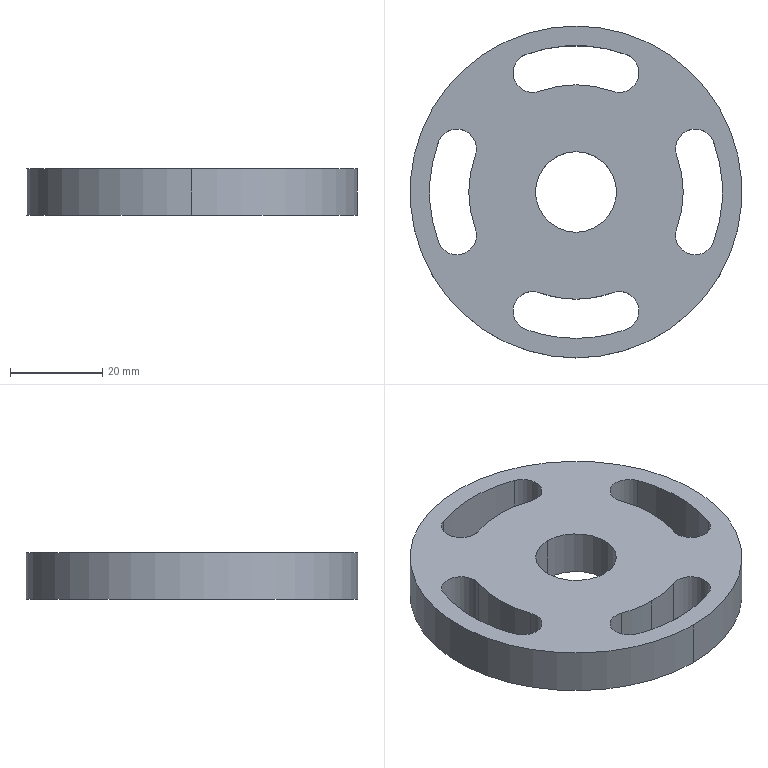NC program | NX | posted with a generic post | part box 72 x 72 x 10 mm
Lines 1 to 834 of 21342:
N10 G17 G21 G94 G90
(ZLEVEL_PROFILE , TOOL : D6C)
N12 T06 M6
N14 G54
N16 G17 G0 G90 X-6.398 Y25.475 S4000 M3
N18 G43 Z30. H6
N20 Z1.5
N22 G94 G1 X-4.667 Y25.852 Z1.407 F1800.
N24 X-2.81 Y26.119 Z1.309
N26 X-0.938 Y26.253 Z1.21
N28 X0.938 Z1.112
N30 X2.81 Y26.119 Z1.014
N32 X4.667 Y25.852 Z0.915
N34 X6.5 Y25.453 Z0.817
N36 X8.3 Y24.924 Z0.719
N38 X9.13 Y24.622 Z0.673
N40 X9.247 Y24.602 Z0.666
N42 X9.563 Y24.601 Z0.65
N44 X9.967 Y24.725 Z0.628
N46 X10.308 Y24.976 Z0.605
N48 X10.545 Y25.327 Z0.583
N50 X10.651 Y25.736 Z0.561
N52 X10.615 Y26.158 Z0.539
N54 X10.497 Y26.45 Z0.522
N56 X10.275 Y26.74 Z0.503
N58 X9.978 Y26.953 Z0.484
N60 X9.117 Y27.266 Z0.436
N62 X7.074 Y27.866 Z0.325
N64 X4.992 Y28.313 Z0.213
N66 X2.883 Y28.605 Z0.101
N68 X0.758 Y28.74 Z-0.01
N70 X0. Z-0.05
N72 G3 X-9.83 Y27.007 R28.74
N74 X-10.571 Y25.417 R1.24
N76 X-8.981 Y24.676 R1.24
N78 G2 X8.981 Y24.676 R26.26
N80 G3 X10.571 Y25.417 R1.24
N82 X9.83 Y27.007 R1.24
N84 X0. Y28.74 R28.74
N86 G1 X-0.159 Y28.736 Z-0.053
N88 X-0.318 Y28.732 Z-0.056
N90 X-0.477 Y28.728 Z-0.058
N92 X-0.636 Y28.724 Z-0.061
N94 X-0.795 Y28.72 Z-0.064
N96 X-0.954 Y28.716 Z-0.067
N98 X-1.113 Y28.712 Z-0.069
N100 X-1.273 Y28.708 Z-0.072
N102 X-1.432 Y28.704 Z-0.075
N104 X-1.59 Y28.692 Z-0.078
N106 X-1.749 Y28.681 Z-0.081
N108 X-1.908 Y28.669 Z-0.083
N110 X-2.066 Y28.657 Z-0.086
N112 X-2.225 Y28.645 Z-0.089
N114 X-2.384 Y28.633 Z-0.092
N116 X-2.542 Y28.621 Z-0.094
N118 X-2.701 Y28.609 Z-0.097
N120 X-2.86 Y28.597 Z-0.1
N122 G3 X-9.83 Y27.007 R28.74
N124 X-10.571 Y25.417 R1.24
N126 X-8.981 Y24.676 R1.24
N128 G2 X8.981 Y24.676 R26.26
N130 G3 X10.571 Y25.417 R1.24
N132 X9.83 Y27.007 R1.24
N134 X0. Y28.74 R28.74
N136 G1 X-0.159 Y28.736 Z-0.103
N138 X-0.318 Y28.732 Z-0.106
N140 X-0.477 Y28.728 Z-0.108
N142 X-0.636 Y28.724 Z-0.111
N144 X-0.795 Y28.72 Z-0.114
N146 X-0.954 Y28.716 Z-0.117
N148 X-1.113 Y28.712 Z-0.119
N150 X-1.273 Y28.708 Z-0.122
N152 X-1.432 Y28.704 Z-0.125
N154 X-1.59 Y28.692 Z-0.128
N156 X-1.749 Y28.681 Z-0.131
N158 X-1.908 Y28.669 Z-0.133
N160 X-2.066 Y28.657 Z-0.136
N162 X-2.225 Y28.645 Z-0.139
N164 X-2.384 Y28.633 Z-0.142
N166 X-2.542 Y28.621 Z-0.144
N168 X-2.701 Y28.609 Z-0.147
N170 X-2.86 Y28.597 Z-0.15
N172 G3 X-9.83 Y27.007 R28.74
N174 X-10.571 Y25.417 R1.24
N176 X-8.981 Y24.676 R1.24
N178 G2 X8.981 Y24.676 R26.26
N180 G3 X10.571 Y25.417 R1.24
N182 X9.83 Y27.007 R1.24
N184 X0. Y28.74 R28.74
N186 G1 X-0.159 Y28.736 Z-0.153
N188 X-0.318 Y28.732 Z-0.156
N190 X-0.477 Y28.728 Z-0.158
N192 X-0.636 Y28.724 Z-0.161
N194 X-0.795 Y28.72 Z-0.164
N196 X-0.954 Y28.716 Z-0.167
N198 X-1.113 Y28.712 Z-0.169
N200 X-1.273 Y28.708 Z-0.172
N202 X-1.432 Y28.704 Z-0.175
N204 X-1.59 Y28.692 Z-0.178
N206 X-1.749 Y28.681 Z-0.181
N208 X-1.908 Y28.669 Z-0.183
N210 X-2.066 Y28.657 Z-0.186
N212 X-2.225 Y28.645 Z-0.189
N214 X-2.384 Y28.633 Z-0.192
N216 X-2.542 Y28.621 Z-0.194
N218 X-2.701 Y28.609 Z-0.197
N220 X-2.86 Y28.597 Z-0.2
N222 G3 X-9.83 Y27.007 R28.74
N224 X-10.571 Y25.417 R1.24
N226 X-8.981 Y24.676 R1.24
N228 G2 X8.981 Y24.676 R26.26
N230 G3 X10.571 Y25.417 R1.24
N232 X9.83 Y27.007 R1.24
N234 X0. Y28.74 R28.74
N236 G1 X-0.159 Y28.736 Z-0.203
N238 X-0.318 Y28.732 Z-0.206
N240 X-0.477 Y28.728 Z-0.208
N242 X-0.636 Y28.724 Z-0.211
N244 X-0.795 Y28.72 Z-0.214
N246 X-0.954 Y28.716 Z-0.217
N248 X-1.113 Y28.712 Z-0.219
N250 X-1.273 Y28.708 Z-0.222
N252 X-1.432 Y28.704 Z-0.225
N254 X-1.59 Y28.692 Z-0.228
N256 X-1.749 Y28.681 Z-0.231
N258 X-1.908 Y28.669 Z-0.233
N260 X-2.066 Y28.657 Z-0.236
N262 X-2.225 Y28.645 Z-0.239
N264 X-2.384 Y28.633 Z-0.242
N266 X-2.542 Y28.621 Z-0.244
N268 X-2.701 Y28.609 Z-0.247
N270 X-2.86 Y28.597 Z-0.25
N272 G3 X-9.83 Y27.007 R28.74
N274 X-10.571 Y25.417 R1.24
N276 X-8.981 Y24.676 R1.24
N278 G2 X8.981 Y24.676 R26.26
N280 G3 X10.571 Y25.417 R1.24
N282 X9.83 Y27.007 R1.24
N284 X0. Y28.74 R28.74
N286 G1 X-0.159 Y28.736 Z-0.253
N288 X-0.318 Y28.732 Z-0.256
N290 X-0.477 Y28.728 Z-0.258
N292 X-0.636 Y28.724 Z-0.261
N294 X-0.795 Y28.72 Z-0.264
N296 X-0.954 Y28.716 Z-0.267
N298 X-1.113 Y28.712 Z-0.269
N300 X-1.273 Y28.708 Z-0.272
N302 X-1.432 Y28.704 Z-0.275
N304 X-1.59 Y28.692 Z-0.278
N306 X-1.749 Y28.681 Z-0.281
N308 X-1.908 Y28.669 Z-0.283
N310 X-2.066 Y28.657 Z-0.286
N312 X-2.225 Y28.645 Z-0.289
N314 X-2.384 Y28.633 Z-0.292
N316 X-2.542 Y28.621 Z-0.294
N318 X-2.701 Y28.609 Z-0.297
N320 X-2.86 Y28.597 Z-0.3
N322 G3 X-9.83 Y27.007 R28.74
N324 X-10.571 Y25.417 R1.24
N326 X-8.981 Y24.676 R1.24
N328 G2 X8.981 Y24.676 R26.26
N330 G3 X10.571 Y25.417 R1.24
N332 X9.83 Y27.007 R1.24
N334 X0. Y28.74 R28.74
N336 G1 X-0.159 Y28.736 Z-0.303
N338 X-0.318 Y28.732 Z-0.306
N340 X-0.477 Y28.728 Z-0.308
N342 X-0.636 Y28.724 Z-0.311
N344 X-0.795 Y28.72 Z-0.314
N346 X-0.954 Y28.716 Z-0.317
N348 X-1.113 Y28.712 Z-0.319
N350 X-1.273 Y28.708 Z-0.322
N352 X-1.432 Y28.704 Z-0.325
N354 X-1.59 Y28.692 Z-0.328
N356 X-1.749 Y28.681 Z-0.331
N358 X-1.908 Y28.669 Z-0.333
N360 X-2.066 Y28.657 Z-0.336
N362 X-2.225 Y28.645 Z-0.339
N364 X-2.384 Y28.633 Z-0.342
N366 X-2.542 Y28.621 Z-0.344
N368 X-2.701 Y28.609 Z-0.347
N370 X-2.86 Y28.597 Z-0.35
N372 G3 X-9.83 Y27.007 R28.74
N374 X-10.571 Y25.417 R1.24
N376 X-8.981 Y24.676 R1.24
N378 G2 X8.981 Y24.676 R26.26
N380 G3 X10.571 Y25.417 R1.24
N382 X9.83 Y27.007 R1.24
N384 X0. Y28.74 R28.74
N386 G1 X-0.159 Y28.736 Z-0.353
N388 X-0.318 Y28.732 Z-0.356
N390 X-0.477 Y28.728 Z-0.358
N392 X-0.636 Y28.724 Z-0.361
N394 X-0.795 Y28.72 Z-0.364
N396 X-0.954 Y28.716 Z-0.367
N398 X-1.113 Y28.712 Z-0.369
N400 X-1.273 Y28.708 Z-0.372
N402 X-1.432 Y28.704 Z-0.375
N404 X-1.59 Y28.692 Z-0.378
N406 X-1.749 Y28.681 Z-0.381
N408 X-1.908 Y28.669 Z-0.383
N410 X-2.066 Y28.657 Z-0.386
N412 X-2.225 Y28.645 Z-0.389
N414 X-2.384 Y28.633 Z-0.392
N416 X-2.542 Y28.621 Z-0.394
N418 X-2.701 Y28.609 Z-0.397
N420 X-2.86 Y28.597 Z-0.4
N422 G3 X-9.83 Y27.007 R28.74
N424 X-10.571 Y25.417 R1.24
N426 X-8.981 Y24.676 R1.24
N428 G2 X8.981 Y24.676 R26.26
N430 G3 X10.571 Y25.417 R1.24
N432 X9.83 Y27.007 R1.24
N434 X0. Y28.74 R28.74
N436 G1 X-0.159 Y28.736 Z-0.403
N438 X-0.318 Y28.732 Z-0.406
N440 X-0.477 Y28.728 Z-0.408
N442 X-0.636 Y28.724 Z-0.411
N444 X-0.795 Y28.72 Z-0.414
N446 X-0.954 Y28.716 Z-0.417
N448 X-1.113 Y28.712 Z-0.419
N450 X-1.273 Y28.708 Z-0.422
N452 X-1.432 Y28.704 Z-0.425
N454 X-1.59 Y28.692 Z-0.428
N456 X-1.749 Y28.681 Z-0.431
N458 X-1.908 Y28.669 Z-0.433
N460 X-2.066 Y28.657 Z-0.436
N462 X-2.225 Y28.645 Z-0.439
N464 X-2.384 Y28.633 Z-0.442
N466 X-2.542 Y28.621 Z-0.444
N468 X-2.701 Y28.609 Z-0.447
N470 X-2.86 Y28.597 Z-0.45
N472 G3 X-9.83 Y27.007 R28.74
N474 X-10.571 Y25.417 R1.24
N476 X-8.981 Y24.676 R1.24
N478 G2 X8.981 Y24.676 R26.26
N480 G3 X10.571 Y25.417 R1.24
N482 X9.83 Y27.007 R1.24
N484 X0. Y28.74 R28.74
N486 G1 X-0.159 Y28.736 Z-0.453
N488 X-0.318 Y28.732 Z-0.456
N490 X-0.477 Y28.728 Z-0.458
N492 X-0.636 Y28.724 Z-0.461
N494 X-0.795 Y28.72 Z-0.464
N496 X-0.954 Y28.716 Z-0.467
N498 X-1.113 Y28.712 Z-0.469
N500 X-1.273 Y28.708 Z-0.472
N502 X-1.432 Y28.704 Z-0.475
N504 X-1.59 Y28.692 Z-0.478
N506 X-1.749 Y28.681 Z-0.481
N508 X-1.908 Y28.669 Z-0.483
N510 X-2.066 Y28.657 Z-0.486
N512 X-2.225 Y28.645 Z-0.489
N514 X-2.384 Y28.633 Z-0.492
N516 X-2.542 Y28.621 Z-0.494
N518 X-2.701 Y28.609 Z-0.497
N520 X-2.86 Y28.597 Z-0.5
N522 G3 X-9.83 Y27.007 R28.74
N524 X-10.571 Y25.417 R1.24
N526 X-8.981 Y24.676 R1.24
N528 G2 X8.981 Y24.676 R26.26
N530 G3 X10.571 Y25.417 R1.24
N532 X9.83 Y27.007 R1.24
N534 X0. Y28.74 R28.74
N536 G1 X-0.159 Y28.736 Z-0.503
N538 X-0.318 Y28.732 Z-0.506
N540 X-0.477 Y28.728 Z-0.508
N542 X-0.636 Y28.724 Z-0.511
N544 X-0.795 Y28.72 Z-0.514
N546 X-0.954 Y28.716 Z-0.517
N548 X-1.113 Y28.712 Z-0.519
N550 X-1.273 Y28.708 Z-0.522
N552 X-1.432 Y28.704 Z-0.525
N554 X-1.59 Y28.692 Z-0.528
N556 X-1.749 Y28.681 Z-0.531
N558 X-1.908 Y28.669 Z-0.533
N560 X-2.066 Y28.657 Z-0.536
N562 X-2.225 Y28.645 Z-0.539
N564 X-2.384 Y28.633 Z-0.542
N566 X-2.542 Y28.621 Z-0.544
N568 X-2.701 Y28.609 Z-0.547
N570 X-2.86 Y28.597 Z-0.55
N572 G3 X-9.83 Y27.007 R28.74
N574 X-10.571 Y25.417 R1.24
N576 X-8.981 Y24.676 R1.24
N578 G2 X8.981 Y24.676 R26.26
N580 G3 X10.571 Y25.417 R1.24
N582 X9.83 Y27.007 R1.24
N584 X0. Y28.74 R28.74
N586 G1 X-0.159 Y28.736 Z-0.553
N588 X-0.318 Y28.732 Z-0.556
N590 X-0.477 Y28.728 Z-0.558
N592 X-0.636 Y28.724 Z-0.561
N594 X-0.795 Y28.72 Z-0.564
N596 X-0.954 Y28.716 Z-0.567
N598 X-1.113 Y28.712 Z-0.569
N600 X-1.273 Y28.708 Z-0.572
N602 X-1.432 Y28.704 Z-0.575
N604 X-1.59 Y28.692 Z-0.578
N606 X-1.749 Y28.681 Z-0.581
N608 X-1.908 Y28.669 Z-0.583
N610 X-2.066 Y28.657 Z-0.586
N612 X-2.225 Y28.645 Z-0.589
N614 X-2.384 Y28.633 Z-0.592
N616 X-2.542 Y28.621 Z-0.594
N618 X-2.701 Y28.609 Z-0.597
N620 X-2.86 Y28.597 Z-0.6
N622 G3 X-9.83 Y27.007 R28.74
N624 X-10.571 Y25.417 R1.24
N626 X-8.981 Y24.676 R1.24
N628 G2 X8.981 Y24.676 R26.26
N630 G3 X10.571 Y25.417 R1.24
N632 X9.83 Y27.007 R1.24
N634 X0. Y28.74 R28.74
N636 G1 X-0.159 Y28.736 Z-0.603
N638 X-0.318 Y28.732 Z-0.606
N640 X-0.477 Y28.728 Z-0.608
N642 X-0.636 Y28.724 Z-0.611
N644 X-0.795 Y28.72 Z-0.614
N646 X-0.954 Y28.716 Z-0.617
N648 X-1.113 Y28.712 Z-0.619
N650 X-1.273 Y28.708 Z-0.622
N652 X-1.432 Y28.704 Z-0.625
N654 X-1.59 Y28.692 Z-0.628
N656 X-1.749 Y28.681 Z-0.631
N658 X-1.908 Y28.669 Z-0.633
N660 X-2.066 Y28.657 Z-0.636
N662 X-2.225 Y28.645 Z-0.639
N664 X-2.384 Y28.633 Z-0.642
N666 X-2.542 Y28.621 Z-0.644
N668 X-2.701 Y28.609 Z-0.647
N670 X-2.86 Y28.597 Z-0.65
N672 G3 X-9.83 Y27.007 R28.74
N674 X-10.571 Y25.417 R1.24
N676 X-8.981 Y24.676 R1.24
N678 G2 X8.981 Y24.676 R26.26
N680 G3 X10.571 Y25.417 R1.24
N682 X9.83 Y27.007 R1.24
N684 X0. Y28.74 R28.74
N686 G1 X-0.159 Y28.736 Z-0.653
N688 X-0.318 Y28.732 Z-0.656
N690 X-0.477 Y28.728 Z-0.658
N692 X-0.636 Y28.724 Z-0.661
N694 X-0.795 Y28.72 Z-0.664
N696 X-0.954 Y28.716 Z-0.667
N698 X-1.113 Y28.712 Z-0.669
N700 X-1.273 Y28.708 Z-0.672
N702 X-1.432 Y28.704 Z-0.675
N704 X-1.59 Y28.692 Z-0.678
N706 X-1.749 Y28.681 Z-0.681
N708 X-1.908 Y28.669 Z-0.683
N710 X-2.066 Y28.657 Z-0.686
N712 X-2.225 Y28.645 Z-0.689
N714 X-2.384 Y28.633 Z-0.692
N716 X-2.542 Y28.621 Z-0.694
N718 X-2.701 Y28.609 Z-0.697
N720 X-2.86 Y28.597 Z-0.7
N722 G3 X-9.83 Y27.007 R28.74
N724 X-10.571 Y25.417 R1.24
N726 X-8.981 Y24.676 R1.24
N728 G2 X8.981 Y24.676 R26.26
N730 G3 X10.571 Y25.417 R1.24
N732 X9.83 Y27.007 R1.24
N734 X0. Y28.74 R28.74
N736 G1 X-0.159 Y28.736 Z-0.703
N738 X-0.318 Y28.732 Z-0.706
N740 X-0.477 Y28.728 Z-0.708
N742 X-0.636 Y28.724 Z-0.711
N744 X-0.795 Y28.72 Z-0.714
N746 X-0.954 Y28.716 Z-0.717
N748 X-1.113 Y28.712 Z-0.719
N750 X-1.273 Y28.708 Z-0.722
N752 X-1.432 Y28.704 Z-0.725
N754 X-1.59 Y28.692 Z-0.728
N756 X-1.749 Y28.681 Z-0.731
N758 X-1.908 Y28.669 Z-0.733
N760 X-2.066 Y28.657 Z-0.736
N762 X-2.225 Y28.645 Z-0.739
N764 X-2.384 Y28.633 Z-0.742
N766 X-2.542 Y28.621 Z-0.744
N768 X-2.701 Y28.609 Z-0.747
N770 X-2.86 Y28.597 Z-0.75
N772 G3 X-9.83 Y27.007 R28.74
N774 X-10.571 Y25.417 R1.24
N776 X-8.981 Y24.676 R1.24
N778 G2 X8.981 Y24.676 R26.26
N780 G3 X10.571 Y25.417 R1.24
N782 X9.83 Y27.007 R1.24
N784 X0. Y28.74 R28.74
N786 G1 X-0.159 Y28.736 Z-0.753
N788 X-0.318 Y28.732 Z-0.756
N790 X-0.477 Y28.728 Z-0.758
N792 X-0.636 Y28.724 Z-0.761
N794 X-0.795 Y28.72 Z-0.764
N796 X-0.954 Y28.716 Z-0.767
N798 X-1.113 Y28.712 Z-0.769
N800 X-1.273 Y28.708 Z-0.772
N802 X-1.432 Y28.704 Z-0.775
N804 X-1.59 Y28.692 Z-0.778
N806 X-1.749 Y28.681 Z-0.781
N808 X-1.908 Y28.669 Z-0.783
N810 X-2.066 Y28.657 Z-0.786
N812 X-2.225 Y28.645 Z-0.789
N814 X-2.384 Y28.633 Z-0.792
N816 X-2.542 Y28.621 Z-0.794
N818 X-2.701 Y28.609 Z-0.797
N820 X-2.86 Y28.597 Z-0.8
N822 G3 X-9.83 Y27.007 R28.74
N824 X-10.571 Y25.417 R1.24
N826 X-8.981 Y24.676 R1.24
N828 G2 X8.981 Y24.676 R26.26
N830 G3 X10.571 Y25.417 R1.24
N832 X9.83 Y27.007 R1.24
N834 X0. Y28.74 R28.74
N836 G1 X-0.159 Y28.736 Z-0.803
N838 X-0.318 Y28.732 Z-0.806
N840 X-0.477 Y28.728 Z-0.808
N842 X-0.636 Y28.724 Z-0.811
N844 X-0.795 Y28.72 Z-0.814
N846 X-0.954 Y28.716 Z-0.817
N848 X-1.113 Y28.712 Z-0.819
N850 X-1.273 Y28.708 Z-0.822
N852 X-1.432 Y28.704 Z-0.825
N854 X-1.59 Y28.692 Z-0.828
N856 X-1.749 Y28.681 Z-0.831
N858 X-1.908 Y28.669 Z-0.833
N860 X-2.066 Y28.657 Z-0.836
N862 X-2.225 Y28.645 Z-0.839
N864 X-2.384 Y28.633 Z-0.842
N866 X-2.542 Y28.621 Z-0.844
N868 X-2.701 Y28.609 Z-0.847
N870 X-2.86 Y28.597 Z-0.85
N872 G3 X-9.83 Y27.007 R28.74
N874 X-10.571 Y25.417 R1.24
N876 X-8.981 Y24.676 R1.24
N878 G2 X8.981 Y24.676 R26.26
N880 G3 X10.571 Y25.417 R1.24
N882 X9.83 Y27.007 R1.24
N884 X0. Y28.74 R28.74
N886 G1 X-0.159 Y28.736 Z-0.853
N888 X-0.318 Y28.732 Z-0.856
N890 X-0.477 Y28.728 Z-0.858
N892 X-0.636 Y28.724 Z-0.861
N894 X-0.795 Y28.72 Z-0.864
N896 X-0.954 Y28.716 Z-0.867
N898 X-1.113 Y28.712 Z-0.869
N900 X-1.273 Y28.708 Z-0.872
N902 X-1.432 Y28.704 Z-0.875
N904 X-1.59 Y28.692 Z-0.878
N906 X-1.749 Y28.681 Z-0.881
N908 X-1.908 Y28.669 Z-0.883
N910 X-2.066 Y28.657 Z-0.886
N912 X-2.225 Y28.645 Z-0.889
N914 X-2.384 Y28.633 Z-0.892
N916 X-2.542 Y28.621 Z-0.894
N918 X-2.701 Y28.609 Z-0.897
N920 X-2.86 Y28.597 Z-0.9
N922 G3 X-9.83 Y27.007 R28.74
N924 X-10.571 Y25.417 R1.24
N926 X-8.981 Y24.676 R1.24
N928 G2 X8.981 Y24.676 R26.26
N930 G3 X10.571 Y25.417 R1.24
N932 X9.83 Y27.007 R1.24
N934 X0. Y28.74 R28.74
N936 G1 X-0.159 Y28.736 Z-0.903
N938 X-0.318 Y28.732 Z-0.906
N940 X-0.477 Y28.728 Z-0.908
N942 X-0.636 Y28.724 Z-0.911
N944 X-0.795 Y28.72 Z-0.914
N946 X-0.954 Y28.716 Z-0.917
N948 X-1.113 Y28.712 Z-0.919
N950 X-1.273 Y28.708 Z-0.922
N952 X-1.432 Y28.704 Z-0.925
N954 X-1.59 Y28.692 Z-0.928
N956 X-1.749 Y28.681 Z-0.931
N958 X-1.908 Y28.669 Z-0.933
N960 X-2.066 Y28.657 Z-0.936
N962 X-2.225 Y28.645 Z-0.939
N964 X-2.384 Y28.633 Z-0.942
N966 X-2.542 Y28.621 Z-0.944
N968 X-2.701 Y28.609 Z-0.947
N970 X-2.86 Y28.597 Z-0.95
N972 G3 X-9.83 Y27.007 R28.74
N974 X-10.571 Y25.417 R1.24
N976 X-8.981 Y24.676 R1.24
N978 G2 X8.981 Y24.676 R26.26
N980 G3 X10.571 Y25.417 R1.24
N982 X9.83 Y27.007 R1.24
N984 X0. Y28.74 R28.74
N986 G1 X-0.159 Y28.736 Z-0.953
N988 X-0.318 Y28.732 Z-0.956
N990 X-0.477 Y28.728 Z-0.958
N992 X-0.636 Y28.724 Z-0.961
N994 X-0.795 Y28.72 Z-0.964
N996 X-0.954 Y28.716 Z-0.967
N998 X-1.113 Y28.712 Z-0.969
N1000 X-1.273 Y28.708 Z-0.972
N1002 X-1.432 Y28.704 Z-0.975
N1004 X-1.59 Y28.692 Z-0.978
N1006 X-1.749 Y28.681 Z-0.981
N1008 X-1.908 Y28.669 Z-0.983
N1010 X-2.066 Y28.657 Z-0.986
N1012 X-2.225 Y28.645 Z-0.989
N1014 X-2.384 Y28.633 Z-0.992
N1016 X-2.542 Y28.621 Z-0.994
N1018 X-2.701 Y28.609 Z-0.997
N1020 X-2.86 Y28.597 Z-1.
N1022 G3 X-9.83 Y27.007 R28.74
N1024 X-10.571 Y25.417 R1.24
N1026 X-8.981 Y24.676 R1.24
N1028 G2 X8.981 Y24.676 R26.26
N1030 G3 X10.571 Y25.417 R1.24
N1032 X9.83 Y27.007 R1.24
N1034 X0. Y28.74 R28.74
N1036 G1 X-0.159 Y28.736 Z-1.003
N1038 X-0.318 Y28.732 Z-1.006
N1040 X-0.477 Y28.728 Z-1.008
N1042 X-0.636 Y28.724 Z-1.011
N1044 X-0.795 Y28.72 Z-1.014
N1046 X-0.954 Y28.716 Z-1.017
N1048 X-1.113 Y28.712 Z-1.019
N1050 X-1.273 Y28.708 Z-1.022
N1052 X-1.432 Y28.704 Z-1.025
N1054 X-1.59 Y28.692 Z-1.028
N1056 X-1.749 Y28.681 Z-1.031
N1058 X-1.908 Y28.669 Z-1.033
N1060 X-2.066 Y28.657 Z-1.036
N1062 X-2.225 Y28.645 Z-1.039
N1064 X-2.384 Y28.633 Z-1.042
N1066 X-2.542 Y28.621 Z-1.044
N1068 X-2.701 Y28.609 Z-1.047
N1070 X-2.86 Y28.597 Z-1.05
N1072 G3 X-9.83 Y27.007 R28.74
N1074 X-10.571 Y25.417 R1.24
N1076 X-8.981 Y24.676 R1.24
N1078 G2 X8.981 Y24.676 R26.26
N1080 G3 X10.571 Y25.417 R1.24
N1082 X9.83 Y27.007 R1.24
N1084 X0. Y28.74 R28.74
N1086 G1 X-0.159 Y28.736 Z-1.053
N1088 X-0.318 Y28.732 Z-1.056
N1090 X-0.477 Y28.728 Z-1.058
N1092 X-0.636 Y28.724 Z-1.061
N1094 X-0.795 Y28.72 Z-1.064
N1096 X-0.954 Y28.716 Z-1.067
N1098 X-1.113 Y28.712 Z-1.069
N1100 X-1.273 Y28.708 Z-1.072
N1102 X-1.432 Y28.704 Z-1.075
N1104 X-1.59 Y28.692 Z-1.078
N1106 X-1.749 Y28.681 Z-1.081
N1108 X-1.908 Y28.669 Z-1.083
N1110 X-2.066 Y28.657 Z-1.086
N1112 X-2.225 Y28.645 Z-1.089
N1114 X-2.384 Y28.633 Z-1.092
N1116 X-2.542 Y28.621 Z-1.094
N1118 X-2.701 Y28.609 Z-1.097
N1120 X-2.86 Y28.597 Z-1.1
N1122 G3 X-9.83 Y27.007 R28.74
N1124 X-10.571 Y25.417 R1.24
N1126 X-8.981 Y24.676 R1.24
N1128 G2 X8.981 Y24.676 R26.26
N1130 G3 X10.571 Y25.417 R1.24
N1132 X9.83 Y27.007 R1.24
N1134 X0. Y28.74 R28.74
N1136 G1 X-0.159 Y28.736 Z-1.103
N1138 X-0.318 Y28.732 Z-1.106
N1140 X-0.477 Y28.728 Z-1.108
N1142 X-0.636 Y28.724 Z-1.111
N1144 X-0.795 Y28.72 Z-1.114
N1146 X-0.954 Y28.716 Z-1.117
N1148 X-1.113 Y28.712 Z-1.119
N1150 X-1.273 Y28.708 Z-1.122
N1152 X-1.432 Y28.704 Z-1.125
N1154 X-1.59 Y28.692 Z-1.128
N1156 X-1.749 Y28.681 Z-1.131
N1158 X-1.908 Y28.669 Z-1.133
N1160 X-2.066 Y28.657 Z-1.136
N1162 X-2.225 Y28.645 Z-1.139
N1164 X-2.384 Y28.633 Z-1.142
N1166 X-2.542 Y28.621 Z-1.144
N1168 X-2.701 Y28.609 Z-1.147
N1170 X-2.86 Y28.597 Z-1.15
N1172 G3 X-9.83 Y27.007 R28.74
N1174 X-10.571 Y25.417 R1.24
N1176 X-8.981 Y24.676 R1.24
N1178 G2 X8.981 Y24.676 R26.26
N1180 G3 X10.571 Y25.417 R1.24
N1182 X9.83 Y27.007 R1.24
N1184 X0. Y28.74 R28.74
N1186 G1 X-0.159 Y28.736 Z-1.153
N1188 X-0.318 Y28.732 Z-1.156
N1190 X-0.477 Y28.728 Z-1.158
N1192 X-0.636 Y28.724 Z-1.161
N1194 X-0.795 Y28.72 Z-1.164
N1196 X-0.954 Y28.716 Z-1.167
N1198 X-1.113 Y28.712 Z-1.169
N1200 X-1.273 Y28.708 Z-1.172
N1202 X-1.432 Y28.704 Z-1.175
N1204 X-1.59 Y28.692 Z-1.178
N1206 X-1.749 Y28.681 Z-1.181
N1208 X-1.908 Y28.669 Z-1.183
N1210 X-2.066 Y28.657 Z-1.186
N1212 X-2.225 Y28.645 Z-1.189
N1214 X-2.384 Y28.633 Z-1.192
N1216 X-2.542 Y28.621 Z-1.194
N1218 X-2.701 Y28.609 Z-1.197
N1220 X-2.86 Y28.597 Z-1.2
N1222 G3 X-9.83 Y27.007 R28.74
N1224 X-10.571 Y25.417 R1.24
N1226 X-8.981 Y24.676 R1.24
N1228 G2 X8.981 Y24.676 R26.26
N1230 G3 X10.571 Y25.417 R1.24
N1232 X9.83 Y27.007 R1.24
N1234 X0. Y28.74 R28.74
N1236 G1 X-0.159 Y28.736 Z-1.203
N1238 X-0.318 Y28.732 Z-1.206
N1240 X-0.477 Y28.728 Z-1.208
N1242 X-0.636 Y28.724 Z-1.211
N1244 X-0.795 Y28.72 Z-1.214
N1246 X-0.954 Y28.716 Z-1.217
N1248 X-1.113 Y28.712 Z-1.219
N1250 X-1.273 Y28.708 Z-1.222
N1252 X-1.432 Y28.704 Z-1.225
N1254 X-1.59 Y28.692 Z-1.228
N1256 X-1.749 Y28.681 Z-1.231
N1258 X-1.908 Y28.669 Z-1.233
N1260 X-2.066 Y28.657 Z-1.236
N1262 X-2.225 Y28.645 Z-1.239
N1264 X-2.384 Y28.633 Z-1.242
N1266 X-2.542 Y28.621 Z-1.244
N1268 X-2.701 Y28.609 Z-1.247
N1270 X-2.86 Y28.597 Z-1.25
N1272 G3 X-9.83 Y27.007 R28.74
N1274 X-10.571 Y25.417 R1.24
N1276 X-8.981 Y24.676 R1.24
N1278 G2 X8.981 Y24.676 R26.26
N1280 G3 X10.571 Y25.417 R1.24
N1282 X9.83 Y27.007 R1.24
N1284 X0. Y28.74 R28.74
N1286 G1 X-0.159 Y28.736 Z-1.253
N1288 X-0.318 Y28.732 Z-1.256
N1290 X-0.477 Y28.728 Z-1.258
N1292 X-0.636 Y28.724 Z-1.261
N1294 X-0.795 Y28.72 Z-1.264
N1296 X-0.954 Y28.716 Z-1.267
N1298 X-1.113 Y28.712 Z-1.269
N1300 X-1.273 Y28.708 Z-1.272
N1302 X-1.432 Y28.704 Z-1.275
N1304 X-1.59 Y28.692 Z-1.278
N1306 X-1.749 Y28.681 Z-1.281
N1308 X-1.908 Y28.669 Z-1.283
N1310 X-2.066 Y28.657 Z-1.286
N1312 X-2.225 Y28.645 Z-1.289
N1314 X-2.384 Y28.633 Z-1.292
N1316 X-2.542 Y28.621 Z-1.294
N1318 X-2.701 Y28.609 Z-1.297
N1320 X-2.86 Y28.597 Z-1.3
N1322 G3 X-9.83 Y27.007 R28.74
N1324 X-10.571 Y25.417 R1.24
N1326 X-8.981 Y24.676 R1.24
N1328 G2 X8.981 Y24.676 R26.26
N1330 G3 X10.571 Y25.417 R1.24
N1332 X9.83 Y27.007 R1.24
N1334 X0. Y28.74 R28.74
N1336 G1 X-0.159 Y28.736 Z-1.303
N1338 X-0.318 Y28.732 Z-1.306
N1340 X-0.477 Y28.728 Z-1.308
N1342 X-0.636 Y28.724 Z-1.311
N1344 X-0.795 Y28.72 Z-1.314
N1346 X-0.954 Y28.716 Z-1.317
N1348 X-1.113 Y28.712 Z-1.319
N1350 X-1.273 Y28.708 Z-1.322
N1352 X-1.432 Y28.704 Z-1.325
N1354 X-1.59 Y28.692 Z-1.328
N1356 X-1.749 Y28.681 Z-1.331
N1358 X-1.908 Y28.669 Z-1.333
N1360 X-2.066 Y28.657 Z-1.336
N1362 X-2.225 Y28.645 Z-1.339
N1364 X-2.384 Y28.633 Z-1.342
N1366 X-2.542 Y28.621 Z-1.344
N1368 X-2.701 Y28.609 Z-1.347
N1370 X-2.86 Y28.597 Z-1.35
N1372 G3 X-9.83 Y27.007 R28.74
N1374 X-10.571 Y25.417 R1.24
N1376 X-8.981 Y24.676 R1.24
N1378 G2 X8.981 Y24.676 R26.26
N1380 G3 X10.571 Y25.417 R1.24
N1382 X9.83 Y27.007 R1.24
N1384 X0. Y28.74 R28.74
N1386 G1 X-0.159 Y28.736 Z-1.353
N1388 X-0.318 Y28.732 Z-1.356
N1390 X-0.477 Y28.728 Z-1.358
N1392 X-0.636 Y28.724 Z-1.361
N1394 X-0.795 Y28.72 Z-1.364
N1396 X-0.954 Y28.716 Z-1.367
N1398 X-1.113 Y28.712 Z-1.369
N1400 X-1.273 Y28.708 Z-1.372
N1402 X-1.432 Y28.704 Z-1.375
N1404 X-1.59 Y28.692 Z-1.378
N1406 X-1.749 Y28.681 Z-1.381
N1408 X-1.908 Y28.669 Z-1.383
N1410 X-2.066 Y28.657 Z-1.386
N1412 X-2.225 Y28.645 Z-1.389
N1414 X-2.384 Y28.633 Z-1.392
N1416 X-2.542 Y28.621 Z-1.394
N1418 X-2.701 Y28.609 Z-1.397
N1420 X-2.86 Y28.597 Z-1.4
N1422 G3 X-9.83 Y27.007 R28.74
N1424 X-10.571 Y25.417 R1.24
N1426 X-8.981 Y24.676 R1.24
N1428 G2 X8.981 Y24.676 R26.26
N1430 G3 X10.571 Y25.417 R1.24
N1432 X9.83 Y27.007 R1.24
N1434 X0. Y28.74 R28.74
N1436 G1 X-0.159 Y28.736 Z-1.403
N1438 X-0.318 Y28.732 Z-1.406
N1440 X-0.477 Y28.728 Z-1.408
N1442 X-0.636 Y28.724 Z-1.411
N1444 X-0.795 Y28.72 Z-1.414
N1446 X-0.954 Y28.716 Z-1.417
N1448 X-1.113 Y28.712 Z-1.419
N1450 X-1.273 Y28.708 Z-1.422
N1452 X-1.432 Y28.704 Z-1.425
N1454 X-1.59 Y28.692 Z-1.428
N1456 X-1.749 Y28.681 Z-1.431
N1458 X-1.908 Y28.669 Z-1.433
N1460 X-2.066 Y28.657 Z-1.436
N1462 X-2.225 Y28.645 Z-1.439
N1464 X-2.384 Y28.633 Z-1.442
N1466 X-2.542 Y28.621 Z-1.444
N1468 X-2.701 Y28.609 Z-1.447
N1470 X-2.86 Y28.597 Z-1.45
N1472 G3 X-9.83 Y27.007 R28.74
N1474 X-10.571 Y25.417 R1.24
N1476 X-8.981 Y24.676 R1.24
N1478 G2 X8.981 Y24.676 R26.26
N1480 G3 X10.571 Y25.417 R1.24
N1482 X9.83 Y27.007 R1.24
N1484 X0. Y28.74 R28.74
N1486 G1 X-0.159 Y28.736 Z-1.453
N1488 X-0.318 Y28.732 Z-1.456
N1490 X-0.477 Y28.728 Z-1.458
N1492 X-0.636 Y28.724 Z-1.461
N1494 X-0.795 Y28.72 Z-1.464
N1496 X-0.954 Y28.716 Z-1.467
N1498 X-1.113 Y28.712 Z-1.469
N1500 X-1.273 Y28.708 Z-1.472
N1502 X-1.432 Y28.704 Z-1.475
N1504 X-1.59 Y28.692 Z-1.478
N1506 X-1.749 Y28.681 Z-1.481
N1508 X-1.908 Y28.669 Z-1.483
N1510 X-2.066 Y28.657 Z-1.486
N1512 X-2.225 Y28.645 Z-1.489
N1514 X-2.384 Y28.633 Z-1.492
N1516 X-2.542 Y28.621 Z-1.494
N1518 X-2.701 Y28.609 Z-1.497
N1520 X-2.86 Y28.597 Z-1.5
N1522 G3 X-9.83 Y27.007 R28.74
N1524 X-10.571 Y25.417 R1.24
N1526 X-8.981 Y24.676 R1.24
N1528 G2 X8.981 Y24.676 R26.26
N1530 G3 X10.571 Y25.417 R1.24
N1532 X9.83 Y27.007 R1.24
N1534 X0. Y28.74 R28.74
N1536 G1 X-0.159 Y28.736 Z-1.503
N1538 X-0.318 Y28.732 Z-1.506
N1540 X-0.477 Y28.728 Z-1.508
N1542 X-0.636 Y28.724 Z-1.511
N1544 X-0.795 Y28.72 Z-1.514
N1546 X-0.954 Y28.716 Z-1.517
N1548 X-1.113 Y28.712 Z-1.519
N1550 X-1.273 Y28.708 Z-1.522
N1552 X-1.432 Y28.704 Z-1.525
N1554 X-1.59 Y28.692 Z-1.528
N1556 X-1.749 Y28.681 Z-1.531
N1558 X-1.908 Y28.669 Z-1.533
N1560 X-2.066 Y28.657 Z-1.536
N1562 X-2.225 Y28.645 Z-1.539
N1564 X-2.384 Y28.633 Z-1.542
N1566 X-2.542 Y28.621 Z-1.544
N1568 X-2.701 Y28.609 Z-1.547
N1570 X-2.86 Y28.597 Z-1.55
N1572 G3 X-9.83 Y27.007 R28.74
N1574 X-10.571 Y25.417 R1.24
N1576 X-8.981 Y24.676 R1.24
N1578 G2 X8.981 Y24.676 R26.26
N1580 G3 X10.571 Y25.417 R1.24
N1582 X9.83 Y27.007 R1.24
N1584 X0. Y28.74 R28.74
N1586 G1 X-0.159 Y28.736 Z-1.553
N1588 X-0.318 Y28.732 Z-1.556
N1590 X-0.477 Y28.728 Z-1.558
N1592 X-0.636 Y28.724 Z-1.561
N1594 X-0.795 Y28.72 Z-1.564
N1596 X-0.954 Y28.716 Z-1.567
N1598 X-1.113 Y28.712 Z-1.569
N1600 X-1.273 Y28.708 Z-1.572
N1602 X-1.432 Y28.704 Z-1.575
N1604 X-1.59 Y28.692 Z-1.578
N1606 X-1.749 Y28.681 Z-1.581
N1608 X-1.908 Y28.669 Z-1.583
N1610 X-2.066 Y28.657 Z-1.586
N1612 X-2.225 Y28.645 Z-1.589
N1614 X-2.384 Y28.633 Z-1.592
N1616 X-2.542 Y28.621 Z-1.594
N1618 X-2.701 Y28.609 Z-1.597
N1620 X-2.86 Y28.597 Z-1.6
N1622 G3 X-9.83 Y27.007 R28.74
N1624 X-10.571 Y25.417 R1.24
N1626 X-8.981 Y24.676 R1.24
N1628 G2 X8.981 Y24.676 R26.26
N1630 G3 X10.571 Y25.417 R1.24
N1632 X9.83 Y27.007 R1.24
N1634 X0. Y28.74 R28.74
N1636 G1 X-0.159 Y28.736 Z-1.603
N1638 X-0.318 Y28.732 Z-1.606
N1640 X-0.477 Y28.728 Z-1.608
N1642 X-0.636 Y28.724 Z-1.611
N1644 X-0.795 Y28.72 Z-1.614
N1646 X-0.954 Y28.716 Z-1.617
N1648 X-1.113 Y28.712 Z-1.619
N1650 X-1.273 Y28.708 Z-1.622
N1652 X-1.432 Y28.704 Z-1.625
N1654 X-1.59 Y28.692 Z-1.628
N1656 X-1.749 Y28.681 Z-1.631
N1658 X-1.908 Y28.669 Z-1.633
N1660 X-2.066 Y28.657 Z-1.636
N1662 X-2.225 Y28.645 Z-1.639
N1664 X-2.384 Y28.633 Z-1.642
N1666 X-2.542 Y28.621 Z-1.644